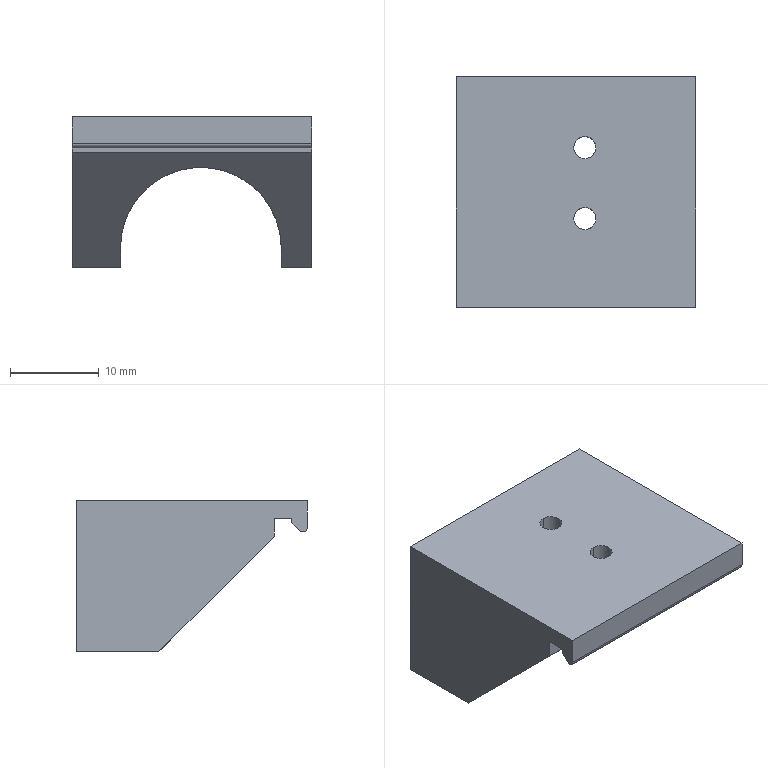NC program | NX | posted with a generic post | part box 27 x 26 x 17 mm
Lines 2084 to 2885 of 22937:
(FIXED_CONTOUR , TOOL : R2)
N4124 T03 M6
N4126 G54
N4128 G17 G0 G90 X-4.906 Y-8.76 S9500 M3
N4130 G43 Z30. H3
N4132 Z-6.
N4134 G94 G1 Z-9.999 F1000.
N4136 G3 X-5.01 Y-8.374 R0.4
N4138 G1 X-5.17 Y-8.214 Z-9.884 F3000.
N4140 X-5.387 Y-7.997 Z-9.717
N4142 X-5.602 Y-7.782 Z-9.538
N4144 X-5.786 Y-7.598 Z-9.376
N4146 X-6.018 Y-7.366 Z-9.151
N4148 X-6.185 Y-7.199 Z-8.977
N4150 X-6.356 Y-7.028 Z-8.783
N4152 X-6.385 Y-6.998 Z-8.747
N4154 X-6.526 Y-6.81 Z-8.578
N4156 X-6.336 Y-7. Z-8.805
N4158 X-6.185 Y-7.151 Z-8.977
N4160 X-6.014 Y-7.322 Z-9.156
N4162 X-5.786 Y-7.55 Z-9.376
N4164 X-5.583 Y-7.752 Z-9.553
N4166 X-5.387 Y-7.949 Z-9.717
N4168 X-5.154 Y-8.182 Z-9.895
N4170 X-4.988 Y-8.348 Z-10.014
N4172 X-4.856 Y-8.48 Z-10.099
N4174 X-4.75 Y-8.551 Z-10.166
N4176 X-4.988 Y-8.313 Z-10.014
N4178 X-5.143 Y-8.158 Z-9.903
N4180 X-5.387 Y-7.914 Z-9.717
N4182 X-5.57 Y-7.731 Z-9.565
N4184 X-5.786 Y-7.515 Z-9.376
N4186 X-6.01 Y-7.29 Z-9.159
N4188 X-6.185 Y-7.116 Z-8.977
N4190 X-6.362 Y-6.938 Z-8.775
N4192 X-6.507 Y-6.794 Z-8.6
N4194 X-6.601 Y-6.7 Z-8.481
N4196 X-6.64 Y-6.643 Z-8.43
N4198 X-6.665 Y-6.603 Z-8.394
N4200 X-6.638 Y-6.63 Z-8.432
N4202 X-6.492 Y-6.776 Z-8.618
N4204 X-6.365 Y-6.903 Z-8.772
N4206 X-6.185 Y-7.084 Z-8.977
N4208 X-6.007 Y-7.261 Z-9.162
N4210 X-5.786 Y-7.482 Z-9.376
N4212 X-5.557 Y-7.711 Z-9.575
N4214 X-5.387 Y-7.881 Z-9.717
N4216 X-5.132 Y-8.136 Z-9.911
N4218 X-4.989 Y-8.279 Z-10.013
N4220 X-4.65 Y-8.618 Z-10.229
N4222 X-4.556 Y-8.679 Z-10.286
N4224 X-4.621 Y-8.615 Z-10.248
N4226 X-4.988 Y-8.247 Z-10.014
N4228 X-5.121 Y-8.114 Z-9.919
N4230 X-5.387 Y-7.848 Z-9.717
N4232 X-5.544 Y-7.691 Z-9.586
N4234 X-5.786 Y-7.449 Z-9.376
N4236 X-6.004 Y-7.231 Z-9.166
N4238 X-6.185 Y-7.051 Z-8.977
N4240 X-6.368 Y-6.868 Z-8.769
N4242 X-6.478 Y-6.758 Z-8.636
N4244 X-6.634 Y-6.601 Z-8.438
N4246 X-6.72 Y-6.516 Z-8.316
N4248 X-6.779 Y-6.421 Z-8.231
N4250 X-6.63 Y-6.57 Z-8.443
N4252 X-6.461 Y-6.738 Z-8.656
N4254 X-6.37 Y-6.829 Z-8.766
N4256 X-6.185 Y-7.015 Z-8.977
N4258 X-6.001 Y-7.198 Z-9.169
N4260 X-5.786 Y-7.414 Z-9.376
N4262 X-5.53 Y-7.669 Z-9.598
N4264 X-5.387 Y-7.812 Z-9.717
N4266 X-5.109 Y-8.09 Z-9.927
N4268 X-4.988 Y-8.211 Z-10.014
N4270 X-4.589 Y-8.61 Z-10.267
N4272 X-4.541 Y-8.658 Z-10.293
N4274 X-4.461 Y-8.738 Z-10.341
N4276 X-4.37 Y-8.793 Z-10.392
N4278 X-4.408 Y-8.755 Z-10.371
N4280 X-4.507 Y-8.657 Z-10.312
N4282 X-4.615 Y-8.548 Z-10.252
N4284 X-4.988 Y-8.175 Z-10.014
N4286 X-5.097 Y-8.066 Z-9.936
N4288 X-5.387 Y-7.776 Z-9.717
N4290 X-5.516 Y-7.647 Z-9.61
N4292 X-5.786 Y-7.377 Z-9.376
N4294 X-5.998 Y-7.166 Z-9.173
N4296 X-6.185 Y-6.979 Z-8.977
N4298 X-6.373 Y-6.79 Z-8.762
N4300 X-6.445 Y-6.718 Z-8.676
N4302 X-6.625 Y-6.538 Z-8.449
N4304 X-6.834 Y-6.329 Z-8.152
N4306 X-6.89 Y-6.237 Z-8.072
N4308 X-6.62 Y-6.506 Z-8.455
N4310 X-6.428 Y-6.698 Z-8.696
N4312 X-6.376 Y-6.75 Z-8.759
N4314 X-6.185 Y-6.942 Z-8.977
N4316 X-5.994 Y-7.132 Z-9.176
N4318 X-5.786 Y-7.34 Z-9.376
N4320 X-5.502 Y-7.624 Z-9.622
N4322 X-5.387 Y-7.739 Z-9.717
N4324 X-5.085 Y-8.041 Z-9.945
N4326 X-4.988 Y-8.138 Z-10.014
N4328 X-4.589 Y-8.537 Z-10.267
N4330 X-4.471 Y-8.655 Z-10.332
N4332 X-4.384 Y-8.742 Z-10.384
N4334 X-4.288 Y-8.838 Z-10.435
N4336 X-4.198 Y-8.888 Z-10.483
N4338 X-4.358 Y-8.728 Z-10.398
N4340 X-4.433 Y-8.653 Z-10.353
N4342 X-4.609 Y-8.477 Z-10.255
N4344 X-4.988 Y-8.098 Z-10.014
N4346 X-5.072 Y-8.014 Z-9.954
N4348 X-5.387 Y-7.699 Z-9.717
N4350 X-5.486 Y-7.599 Z-9.635
N4352 X-5.786 Y-7.3 Z-9.376
N4354 X-5.99 Y-7.095 Z-9.18
N4356 X-6.185 Y-6.901 Z-8.977
N4358 X-6.379 Y-6.706 Z-8.755
N4360 X-6.615 Y-6.47 Z-8.462
N4362 X-6.876 Y-6.21 Z-8.093
N4364 X-6.944 Y-6.142 Z-7.989
N4366 X-7.001 Y-6.037 Z-7.898
N4368 X-6.982 Y-6.056 Z-7.93
N4370 X-6.866 Y-6.172 Z-8.107
N4372 X-6.793 Y-6.245 Z-8.208
N4374 X-6.609 Y-6.429 Z-8.469
N4376 X-6.383 Y-6.655 Z-8.751
N4378 X-6.185 Y-6.854 Z-8.977
N4380 X-5.986 Y-7.052 Z-9.185
N4382 X-5.786 Y-7.253 Z-9.376
N4384 X-5.468 Y-7.57 Z-9.65
N4386 X-5.387 Y-7.651 Z-9.717
N4388 X-5.057 Y-7.982 Z-9.965
N4390 X-4.988 Y-8.05 Z-10.014
N4392 X-4.589 Y-8.449 Z-10.267
N4394 X-4.388 Y-8.65 Z-10.378
N4396 X-4.327 Y-8.712 Z-10.414
N4398 X-4.19 Y-8.848 Z-10.487
N4400 X-4.101 Y-8.937 Z-10.529
N4402 X-4.01 Y-8.983 Z-10.573
N4404 X-4.19 Y-8.802 Z-10.487
N4406 X-4.297 Y-8.696 Z-10.43
N4408 X-4.345 Y-8.648 Z-10.402
N4410 X-4.602 Y-8.391 Z-10.259
N4412 X-4.988 Y-8.005 Z-10.014
N4414 X-5.042 Y-7.951 Z-9.976
N4416 X-5.387 Y-7.606 Z-9.718
N4418 X-5.45 Y-7.542 Z-9.665
N4420 X-5.786 Y-7.207 Z-9.377
N4422 X-5.985 Y-7.008 Z-9.186
N4424 X-6.185 Y-6.808 Z-8.977
N4426 X-6.384 Y-6.609 Z-8.75
N4428 X-6.604 Y-6.389 Z-8.477
N4430 X-6.747 Y-6.245 Z-8.272
N4432 X-6.857 Y-6.136 Z-8.121
N4434 X-6.982 Y-6.011 Z-7.93
N4436 X-7.049 Y-5.944 Z-7.818
N4438 X-7.094 Y-5.855 Z-7.742
N4440 X-6.982 Y-5.966 Z-7.93
N4442 X-6.848 Y-6.101 Z-8.135
N4444 X-6.703 Y-6.245 Z-8.335
N4446 X-6.583 Y-6.365 Z-8.503
N4448 X-6.384 Y-6.565 Z-8.75
N4450 X-6.185 Y-6.764 Z-8.977
N4452 X-5.985 Y-6.963 Z-9.186
N4454 X-5.786 Y-7.163 Z-9.377
N4456 X-5.387 Y-7.562 Z-9.718
N4458 X-4.988 Y-7.96 Z-10.014
N4460 X-4.589 Y-8.359 Z-10.267
N4462 X-4.303 Y-8.646 Z-10.425
N4464 X-4.268 Y-8.681 Z-10.445
N4466 X-4.19 Y-8.758 Z-10.487
N4468 X-3.921 Y-9.028 Z-10.616
N4470 X-3.831 Y-9.072 Z-10.656
N4472 X-3.898 Y-9.005 Z-10.627
N4474 X-4.19 Y-8.713 Z-10.487
N4476 X-4.595 Y-8.308 Z-10.263
N4478 X-4.988 Y-7.915 Z-10.015
N4480 X-5.387 Y-7.516 Z-9.718
N4482 X-5.786 Y-7.118 Z-9.377
N4484 X-5.985 Y-6.918 Z-9.186
N4486 X-6.185 Y-6.719 Z-8.977
N4488 X-6.384 Y-6.519 Z-8.751
N4490 X-6.593 Y-6.311 Z-8.491
N4492 X-6.658 Y-6.245 Z-8.398
N4494 X-6.839 Y-6.065 Z-8.148
N4496 X-6.982 Y-5.921 Z-7.93
N4498 X-7.104 Y-5.799 Z-7.725
N4500 X-7.135 Y-5.768 Z-7.666
N4502 X-7.178 Y-5.679 Z-7.589
N4504 X-7.108 Y-5.748 Z-7.717
N4506 X-6.982 Y-5.874 Z-7.93
N4508 X-6.829 Y-6.027 Z-8.162
N4510 X-6.583 Y-6.273 Z-8.503
N4512 X-6.384 Y-6.473 Z-8.751
N4514 X-6.185 Y-6.672 Z-8.978
N4516 X-5.985 Y-6.871 Z-9.186
N4518 X-5.786 Y-7.071 Z-9.377
N4520 X-5.387 Y-7.47 Z-9.718
N4522 X-4.988 Y-7.868 Z-10.015
N4524 X-4.591 Y-8.265 Z-10.265
N4526 X-4.19 Y-8.666 Z-10.486
N4528 X-3.887 Y-8.969 Z-10.631
N4530 X-3.741 Y-9.115 Z-10.695
N4532 X-3.652 Y-9.156 Z-10.732
N4534 X-3.723 Y-9.085 Z-10.701
N4536 X-3.792 Y-9.016 Z-10.674
N4538 X-3.877 Y-8.931 Z-10.636
N4540 X-4.19 Y-8.618 Z-10.486
N4542 X-4.589 Y-8.219 Z-10.267
N4544 X-4.988 Y-7.82 Z-10.015
N4546 X-5.387 Y-7.421 Z-9.718
N4548 X-5.786 Y-7.022 Z-9.377
N4550 X-5.985 Y-6.823 Z-9.186
N4552 X-6.185 Y-6.624 Z-8.978
N4554 X-6.384 Y-6.424 Z-8.751
N4556 X-6.583 Y-6.225 Z-8.503
N4558 X-6.819 Y-5.989 Z-8.177
N4560 X-6.982 Y-5.826 Z-7.93
N4562 X-7.113 Y-5.695 Z-7.709
N4564 X-7.221 Y-5.587 Z-7.509
N4566 X-7.265 Y-5.491 Z-7.428
N4568 X-7.118 Y-5.638 Z-7.701
N4570 X-6.982 Y-5.774 Z-7.93
N4572 X-6.809 Y-5.948 Z-8.193
N4574 X-6.583 Y-6.173 Z-8.503
N4576 X-6.384 Y-6.372 Z-8.751
N4578 X-6.185 Y-6.572 Z-8.978
N4580 X-5.985 Y-6.771 Z-9.187
N4582 X-5.786 Y-6.971 Z-9.377
N4584 X-5.387 Y-7.369 Z-9.718
N4586 X-4.988 Y-7.768 Z-10.015
N4588 X-4.589 Y-8.167 Z-10.267
N4590 X-4.19 Y-8.566 Z-10.487
N4592 X-3.865 Y-8.891 Z-10.641
N4594 X-3.792 Y-8.965 Z-10.674
N4596 X-3.678 Y-9.079 Z-10.719
N4598 X-3.6 Y-9.157 Z-10.753
N4600 X-3.56 Y-9.196 Z-10.769
N4602 X-3.464 Y-9.236 Z-10.805
N4604 X-3.563 Y-9.136 Z-10.767
N4606 X-3.627 Y-9.072 Z-10.739
N4608 X-3.792 Y-8.907 Z-10.674
N4610 X-3.852 Y-8.847 Z-10.647
N4612 X-4.19 Y-8.509 Z-10.487
N4614 X-4.589 Y-8.11 Z-10.267
N4616 X-4.988 Y-7.711 Z-10.015
N4618 X-5.387 Y-7.312 Z-9.718
N4620 X-5.786 Y-6.913 Z-9.377
N4622 X-5.985 Y-6.714 Z-9.187
N4624 X-6.185 Y-6.515 Z-8.978
N4626 X-6.384 Y-6.315 Z-8.751
N4628 X-6.583 Y-6.116 Z-8.504
N4630 X-6.797 Y-5.902 Z-8.21
N4632 X-6.982 Y-5.717 Z-7.93
N4634 X-7.123 Y-5.576 Z-7.691
N4636 X-7.28 Y-5.419 Z-7.402
N4638 X-7.31 Y-5.389 Z-7.34
N4640 X-7.351 Y-5.293 Z-7.256
N4642 X-7.268 Y-5.375 Z-7.424
N4644 X-7.129 Y-5.514 Z-7.682
N4646 X-6.982 Y-5.661 Z-7.93
N4648 X-6.786 Y-5.858 Z-8.227
N4650 X-6.583 Y-6.06 Z-8.504
N4652 X-6.384 Y-6.259 Z-8.752
N4654 X-6.185 Y-6.459 Z-8.978
N4656 X-5.985 Y-6.658 Z-9.187
N4658 X-5.786 Y-6.858 Z-9.378
N4660 X-5.387 Y-7.256 Z-9.719
N4662 X-4.988 Y-7.655 Z-10.015
N4664 X-4.589 Y-8.054 Z-10.267
N4666 X-4.19 Y-8.453 Z-10.487
N4668 X-3.792 Y-8.852 Z-10.674
N4670 X-3.578 Y-9.065 Z-10.758
N4672 X-3.527 Y-9.116 Z-10.781
N4674 X-3.37 Y-9.273 Z-10.84
N4676 X-3.286 Y-9.304 Z-10.869
N4678 X-3.393 Y-9.197 Z-10.832
N4680 X-3.494 Y-9.096 Z-10.794
N4682 X-3.532 Y-9.058 Z-10.777
N4684 X-3.792 Y-8.798 Z-10.674
N4686 X-4.19 Y-8.399 Z-10.487
N4688 X-4.589 Y-8.001 Z-10.267
N4690 X-4.988 Y-7.602 Z-10.015
N4692 X-5.387 Y-7.203 Z-9.719
N4694 X-5.786 Y-6.804 Z-9.378
N4696 X-5.985 Y-6.605 Z-9.187
N4698 X-6.185 Y-6.405 Z-8.979
N4700 X-6.384 Y-6.206 Z-8.752
N4702 X-6.583 Y-6.007 Z-8.504
N4704 X-6.783 Y-5.807 Z-8.232
N4706 X-6.982 Y-5.608 Z-7.93
N4708 X-7.134 Y-5.456 Z-7.674
N4710 X-7.257 Y-5.333 Z-7.445
N4712 X-7.381 Y-5.209 Z-7.193
N4714 X-7.388 Y-5.202 Z-7.179
N4716 X-7.422 Y-5.115 Z-7.106
N4718 X-7.348 Y-5.189 Z-7.262
N4720 X-7.246 Y-5.291 Z-7.466
N4722 X-7.122 Y-5.415 Z-7.693
N4724 X-6.982 Y-5.555 Z-7.931
N4726 X-6.783 Y-5.754 Z-8.232
N4728 X-6.583 Y-5.954 Z-8.504
N4730 X-6.384 Y-6.153 Z-8.752
N4732 X-6.185 Y-6.352 Z-8.979
N4734 X-5.985 Y-6.552 Z-9.188
N4736 X-5.786 Y-6.751 Z-9.378
N4738 X-5.387 Y-7.15 Z-9.719
N4740 X-4.988 Y-7.549 Z-10.016
N4742 X-4.589 Y-7.948 Z-10.268
N4744 X-4.19 Y-8.346 Z-10.487
N4746 X-3.792 Y-8.745 Z-10.674
N4748 X-3.393 Y-9.144 Z-10.832
N4750 X-3.202 Y-9.334 Z-10.898
N4752 X-3.118 Y-9.365 Z-10.927
N4754 X-3.426 Y-9.058 Z-10.819
N4756 X-3.803 Y-8.68 Z-10.669
N4758 X-4.19 Y-8.293 Z-10.487
N4760 X-4.589 Y-7.894 Z-10.268
N4762 X-4.988 Y-7.495 Z-10.016
N4764 X-5.387 Y-7.097 Z-9.719
N4766 X-5.786 Y-6.698 Z-9.378
N4768 X-5.985 Y-6.498 Z-9.188
N4770 X-6.185 Y-6.299 Z-8.979
N4772 X-6.384 Y-6.1 Z-8.752
N4774 X-6.583 Y-5.9 Z-8.505
N4776 X-6.783 Y-5.701 Z-8.232
N4778 X-6.982 Y-5.501 Z-7.931
N4780 X-7.148 Y-5.336 Z-7.649
N4782 X-7.235 Y-5.249 Z-7.488
N4784 X-7.382 Y-5.101 Z-7.191
N4786 X-7.455 Y-5.028 Z-7.033
N4788 X-7.486 Y-4.941 Z-6.958
N4790 X-7.439 Y-4.987 Z-7.069
N4792 X-7.381 Y-5.045 Z-7.193
N4794 X-7.223 Y-5.204 Z-7.51
N4796 X-7.155 Y-5.271 Z-7.635
N4798 X-6.982 Y-5.444 Z-7.931
N4800 X-6.783 Y-5.644 Z-8.233
N4802 X-6.583 Y-5.843 Z-8.505
N4804 X-6.384 Y-6.043 Z-8.752
N4806 X-6.185 Y-6.242 Z-8.979
N4808 X-5.985 Y-6.441 Z-9.188
N4810 X-5.786 Y-6.641 Z-9.379
N4812 X-5.387 Y-7.04 Z-9.719
N4814 X-4.988 Y-7.438 Z-10.016
N4816 X-4.589 Y-7.837 Z-10.268
N4818 X-4.19 Y-8.236 Z-10.487
N4820 X-3.792 Y-8.635 Z-10.674
N4822 X-3.393 Y-9.034 Z-10.832
N4824 X-3.028 Y-9.398 Z-10.958
N4826 X-2.936 Y-9.429 Z-10.989
N4828 X-3.393 Y-8.973 Z-10.832
N4830 X-3.792 Y-8.574 Z-10.674
N4832 X-4.19 Y-8.175 Z-10.487
N4834 X-4.589 Y-7.776 Z-10.268
N4836 X-4.988 Y-7.378 Z-10.016
N4838 X-5.387 Y-6.979 Z-9.72
N4840 X-5.786 Y-6.58 Z-9.379
N4842 X-5.985 Y-6.381 Z-9.188
N4844 X-6.185 Y-6.181 Z-8.979
N4846 X-6.384 Y-5.982 Z-8.753
N4848 X-6.583 Y-5.782 Z-8.505
N4850 X-6.783 Y-5.583 Z-8.233
N4852 X-6.982 Y-5.384 Z-7.931
N4854 X-7.163 Y-5.202 Z-7.621
N4856 X-7.21 Y-5.156 Z-7.535
N4858 X-7.381 Y-4.985 Z-7.193
N4860 X-7.43 Y-4.935 Z-7.088
N4862 X-7.519 Y-4.847 Z-6.878
N4864 X-7.553 Y-4.748 Z-6.795
N4866 X-7.421 Y-4.88 Z-7.109
N4868 X-7.381 Y-4.919 Z-7.193
N4870 X-7.196 Y-5.104 Z-7.561
N4872 X-7.172 Y-5.128 Z-7.606
N4874 X-6.982 Y-5.318 Z-7.932
N4876 X-6.783 Y-5.518 Z-8.233
N4878 X-6.583 Y-5.717 Z-8.506
N4880 X-6.384 Y-5.916 Z-8.753
N4882 X-6.185 Y-6.116 Z-8.98
N4884 X-5.985 Y-6.315 Z-9.189
N4886 X-5.786 Y-6.515 Z-9.379
N4888 X-5.387 Y-6.913 Z-9.72
N4890 X-4.988 Y-7.312 Z-10.017
N4892 X-4.589 Y-7.711 Z-10.268
N4894 X-4.19 Y-8.11 Z-10.488
N4896 X-3.792 Y-8.509 Z-10.674
N4898 X-3.393 Y-8.907 Z-10.832
N4900 X-2.994 Y-9.306 Z-10.969
N4902 X-2.937 Y-9.363 Z-10.986
N4904 X-2.902 Y-9.398 Z-10.998
N4906 X-2.842 Y-9.458 Z-11.015
N4908 X-2.755 Y-9.485 Z-11.038
N4910 X-2.875 Y-9.366 Z-11.006
N4912 X-2.906 Y-9.334 Z-10.995
N4914 X-2.994 Y-9.246 Z-10.969
N4916 X-3.393 Y-8.847 Z-10.832
N4918 X-3.792 Y-8.449 Z-10.674
N4920 X-4.19 Y-8.05 Z-10.488
N4922 X-4.589 Y-7.651 Z-10.269
N4924 X-4.988 Y-7.252 Z-10.017
N4926 X-5.387 Y-6.853 Z-9.72
N4928 X-5.786 Y-6.454 Z-9.379
N4930 X-5.985 Y-6.255 Z-9.189
N4932 X-6.185 Y-6.056 Z-8.98
N4934 X-6.384 Y-5.856 Z-8.753
N4936 X-6.583 Y-5.657 Z-8.506
N4938 X-6.783 Y-5.457 Z-8.234
N4940 X-6.982 Y-5.258 Z-7.932
N4942 X-7.184 Y-5.056 Z-7.585
N4944 X-7.381 Y-4.859 Z-7.194
N4946 X-7.412 Y-4.828 Z-7.128
N4948 X-7.584 Y-4.657 Z-6.719
N4950 X-7.609 Y-4.572 Z-6.647
N4952 X-7.582 Y-4.6 Z-6.724
N4954 X-7.403 Y-4.778 Z-7.146
N4956 X-7.381 Y-4.8 Z-7.194
N4958 X-7.182 Y-5. Z-7.589
N4960 X-6.982 Y-5.199 Z-7.932
N4962 X-6.783 Y-5.399 Z-8.234
N4964 X-6.583 Y-5.598 Z-8.506
N4966 X-6.384 Y-5.797 Z-8.754
N4968 X-6.185 Y-5.997 Z-8.98
N4970 X-5.985 Y-6.196 Z-9.189
N4972 X-5.786 Y-6.396 Z-9.38
N4974 X-5.387 Y-6.794 Z-9.72
N4976 X-4.988 Y-7.193 Z-10.017
N4978 X-4.589 Y-7.592 Z-10.269
N4980 X-4.19 Y-7.991 Z-10.488
N4982 X-3.792 Y-8.39 Z-10.675
N4984 X-3.393 Y-8.789 Z-10.832
N4986 X-2.994 Y-9.187 Z-10.969
N4988 X-2.876 Y-9.305 Z-11.003
N4990 X-2.848 Y-9.334 Z-11.013
N4992 X-2.67 Y-9.511 Z-11.061
N4994 X-2.587 Y-9.536 Z-11.083
N4996 X-2.821 Y-9.303 Z-11.02
N4998 X-2.846 Y-9.277 Z-11.011
N5000 X-2.994 Y-9.129 Z-10.968
N5002 X-3.393 Y-8.731 Z-10.832
N5004 X-3.792 Y-8.332 Z-10.675
N5006 X-4.19 Y-7.933 Z-10.488
N5008 X-4.589 Y-7.534 Z-10.269
N5010 X-4.988 Y-7.135 Z-10.017
N5012 X-5.387 Y-6.736 Z-9.721
N5014 X-5.786 Y-6.338 Z-9.38
N5016 X-5.985 Y-6.138 Z-9.189
N5018 X-6.185 Y-5.939 Z-8.981
N5020 X-6.384 Y-5.739 Z-8.754
N5022 X-6.583 Y-5.54 Z-8.506
N5024 X-6.783 Y-5.341 Z-8.234
N5026 X-6.982 Y-5.141 Z-7.932
N5028 X-7.182 Y-4.942 Z-7.589
N5030 X-7.395 Y-4.729 Z-7.164
N5032 X-7.475 Y-4.649 Z-6.975
N5034 X-7.576 Y-4.548 Z-6.739
N5036 X-7.634 Y-4.489 Z-6.577
N5038 X-7.658 Y-4.408 Z-6.508
N5040 X-7.57 Y-4.496 Z-6.754
N5042 X-7.381 Y-4.685 Z-7.194
N5044 X-7.182 Y-4.885 Z-7.59
N5046 X-6.982 Y-5.084 Z-7.933
N5048 X-6.783 Y-5.283 Z-8.235
N5050 X-6.583 Y-5.483 Z-8.507
N5052 X-6.384 Y-5.682 Z-8.754
N5054 X-6.185 Y-5.882 Z-8.981
N5056 X-5.985 Y-6.081 Z-9.19
N5058 X-5.786 Y-6.28 Z-9.38
N5060 X-5.387 Y-6.679 Z-9.721
N5062 X-4.988 Y-7.078 Z-10.017
N5064 X-4.589 Y-7.477 Z-10.269
N5066 X-4.19 Y-7.876 Z-10.488
N5068 X-3.792 Y-8.274 Z-10.675
N5070 X-3.393 Y-8.673 Z-10.832
N5072 X-2.994 Y-9.072 Z-10.968
N5074 X-2.794 Y-9.272 Z-11.027
N5076 X-2.595 Y-9.471 Z-11.082
N5078 X-2.511 Y-9.556 Z-11.099
N5080 X-2.434 Y-9.575 Z-11.114
N5082 X-2.595 Y-9.413 Z-11.082
N5084 X-2.768 Y-9.241 Z-11.035
N5086 X-2.994 Y-9.015 Z-10.968
N5088 X-3.393 Y-8.616 Z-10.832
N5090 X-3.792 Y-8.217 Z-10.675
N5092 X-4.19 Y-7.818 Z-10.489
N5094 X-4.589 Y-7.419 Z-10.269
N5096 X-4.988 Y-7.021 Z-10.018
N5098 X-5.387 Y-6.622 Z-9.721
N5100 X-5.786 Y-6.223 Z-9.38
N5102 X-5.985 Y-6.024 Z-9.19
N5104 X-6.185 Y-5.824 Z-8.981
N5106 X-6.384 Y-5.625 Z-8.754
N5108 X-6.583 Y-5.425 Z-8.507
N5110 X-6.783 Y-5.226 Z-8.235
N5112 X-6.982 Y-5.026 Z-7.933
N5114 X-7.182 Y-4.827 Z-7.59
N5116 X-7.381 Y-4.628 Z-7.194
N5118 X-7.564 Y-4.444 Z-6.768
N5120 X-7.682 Y-4.327 Z-6.441
N5122 X-7.705 Y-4.246 Z-6.373
N5124 X-7.558 Y-4.392 Z-6.783
N5126 X-7.381 Y-4.57 Z-7.194
N5128 X-7.182 Y-4.769 Z-7.59
N5130 X-6.982 Y-4.969 Z-7.933
N5132 X-6.783 Y-5.168 Z-8.235
N5134 X-6.583 Y-5.368 Z-8.507
N5136 X-6.384 Y-5.567 Z-8.755
N5138 X-6.185 Y-5.766 Z-8.982
N5140 X-5.985 Y-5.966 Z-9.19
N5142 X-5.786 Y-6.165 Z-9.381
N5144 X-5.387 Y-6.564 Z-9.722
N5146 X-4.988 Y-6.963 Z-10.018
N5148 X-4.589 Y-7.362 Z-10.27
N5150 X-4.19 Y-7.76 Z-10.489
N5152 X-3.792 Y-8.159 Z-10.675
N5154 X-3.393 Y-8.558 Z-10.832
N5156 X-2.994 Y-8.957 Z-10.968
N5158 X-2.741 Y-9.21 Z-11.042
N5160 X-2.595 Y-9.356 Z-11.082
N5162 X-2.361 Y-9.59 Z-11.129
N5164 X-2.286 Y-9.604 Z-11.144
N5166 X-2.595 Y-9.295 Z-11.082
N5168 X-2.727 Y-9.164 Z-11.045
N5170 X-2.994 Y-8.896 Z-10.968
N5172 X-3.393 Y-8.497 Z-10.833
N5174 X-3.792 Y-8.099 Z-10.675
N5176 X-4.19 Y-7.7 Z-10.489
N5178 X-4.589 Y-7.301 Z-10.27
N5180 X-4.988 Y-6.902 Z-10.019
N5182 X-5.387 Y-6.503 Z-9.722
N5184 X-5.786 Y-6.105 Z-9.382
N5186 X-5.985 Y-5.905 Z-9.19
N5188 X-6.185 Y-5.706 Z-8.982
N5190 X-6.384 Y-5.506 Z-8.755
N5192 X-6.583 Y-5.307 Z-8.507
N5194 X-6.783 Y-5.108 Z-8.235
N5196 X-6.982 Y-4.908 Z-7.934
N5198 X-7.182 Y-4.709 Z-7.591
N5200 X-7.381 Y-4.509 Z-7.195
N5202 X-7.552 Y-4.338 Z-6.798
N5204 X-7.701 Y-4.189 Z-6.387
N5206 X-7.727 Y-4.164 Z-6.305
N5208 X-7.749 Y-4.078 Z-6.232
N5210 X-7.697 Y-4.129 Z-6.399
N5212 X-7.546 Y-4.281 Z-6.814
N5214 X-7.381 Y-4.446 Z-7.195
N5216 X-7.182 Y-4.645 Z-7.591
N5218 X-6.982 Y-4.845 Z-7.934
N5220 X-6.783 Y-5.044 Z-8.236
N5222 X-6.583 Y-5.243 Z-8.508
N5224 X-6.384 Y-5.443 Z-8.755
N5226 X-6.185 Y-5.642 Z-8.983
N5228 X-5.985 Y-5.842 Z-9.191
N5230 X-5.786 Y-6.041 Z-9.382
N5232 X-5.387 Y-6.44 Z-9.723
N5234 X-4.988 Y-6.839 Z-10.019
N5236 X-4.589 Y-7.237 Z-10.27
N5238 X-4.19 Y-7.636 Z-10.489
N5240 X-3.792 Y-8.035 Z-10.676
N5242 X-3.393 Y-8.434 Z-10.833
N5244 X-2.994 Y-8.833 Z-10.968
N5246 X-2.595 Y-9.231 Z-11.082
N5248 X-2.207 Y-9.62 Z-11.16
N5250 X-2.128 Y-9.632 Z-11.172
N5252 X-2.196 Y-9.563 Z-11.162
N5254 X-2.595 Y-9.164 Z-11.081
N5256 X-2.994 Y-8.766 Z-10.968
N5258 X-3.393 Y-8.367 Z-10.833
N5260 X-3.792 Y-7.968 Z-10.676
N5262 X-4.19 Y-7.569 Z-10.489
N5264 X-4.589 Y-7.17 Z-10.271
N5266 X-4.988 Y-6.772 Z-10.02
N5268 X-5.387 Y-6.373 Z-9.724
N5270 X-5.786 Y-5.974 Z-9.383
N5272 X-5.985 Y-5.775 Z-9.192
N5274 X-6.185 Y-5.575 Z-8.983
N5276 X-6.384 Y-5.376 Z-8.756
N5278 X-6.583 Y-5.176 Z-8.508
N5280 X-6.783 Y-4.977 Z-8.236
N5282 X-6.982 Y-4.778 Z-7.934
N5284 X-7.182 Y-4.578 Z-7.592
N5286 X-7.381 Y-4.379 Z-7.196
N5288 X-7.546 Y-4.214 Z-6.815
N5290 X-7.693 Y-4.066 Z-6.411
N5292 X-7.772 Y-3.988 Z-6.158
N5294 X-7.794 Y-3.893 Z-6.079
N5296 X-7.78 Y-3.907 Z-6.132
N5298 X-7.689 Y-3.997 Z-6.424
N5300 X-7.554 Y-4.133 Z-6.796
N5302 X-7.381 Y-4.305 Z-7.196
N5304 X-7.182 Y-4.505 Z-7.592
N5306 X-6.982 Y-4.704 Z-7.935
N5308 X-6.783 Y-4.904 Z-8.236
N5310 X-6.583 Y-5.103 Z-8.508
N5312 X-6.384 Y-5.302 Z-8.757
N5314 X-6.185 Y-5.502 Z-8.984
N5316 X-5.985 Y-5.701 Z-9.193
N5318 X-5.786 Y-5.901 Z-9.384
N5320 X-5.387 Y-6.299 Z-9.725
N5322 X-4.988 Y-6.698 Z-10.02
N5324 X-4.589 Y-7.097 Z-10.271
N5326 X-4.19 Y-7.496 Z-10.49
N5328 X-3.792 Y-7.895 Z-10.676
N5330 X-3.393 Y-8.293 Z-10.833
N5332 X-2.994 Y-8.692 Z-10.968
N5334 X-2.595 Y-9.091 Z-11.081
N5336 X-2.196 Y-9.49 Z-11.162
N5338 X-2.043 Y-9.643 Z-11.185
N5340 X-1.961 Y-9.655 Z-11.197
N5342 X-2.196 Y-9.419 Z-11.162
N5344 X-2.595 Y-9.02 Z-11.081
N5346 X-2.994 Y-8.622 Z-10.969
N5348 X-3.393 Y-8.223 Z-10.833
N5350 X-3.792 Y-7.824 Z-10.676
N5352 X-4.19 Y-7.425 Z-10.49
N5354 X-4.589 Y-7.026 Z-10.272
N5356 X-4.988 Y-6.628 Z-10.021
N5358 X-5.387 Y-6.229 Z-9.726
N5360 X-5.786 Y-5.83 Z-9.384
N5362 X-5.985 Y-5.631 Z-9.195
N5364 X-6.2 Y-5.415 Z-8.966
N5366 X-6.384 Y-5.232 Z-8.758
N5368 X-6.583 Y-5.032 Z-8.509
N5370 X-6.783 Y-4.833 Z-8.237
N5372 X-6.982 Y-4.634 Z-7.935
N5374 X-7.182 Y-4.434 Z-7.593
N5376 X-7.381 Y-4.235 Z-7.197
N5378 X-7.561 Y-4.055 Z-6.778
N5380 X-7.685 Y-3.931 Z-6.437
N5382 X-7.78 Y-3.836 Z-6.132
N5384 X-7.812 Y-3.803 Z-6.005
N5386 X-7.83 Y-3.717 Z-5.934
N5388 X-7.78 Y-3.767 Z-6.132
N5390 X-7.681 Y-3.866 Z-6.45
N5392 X-7.568 Y-3.979 Z-6.761
N5394 X-7.381 Y-4.166 Z-7.197
N5396 X-7.182 Y-4.365 Z-7.593
N5398 X-6.982 Y-4.565 Z-7.935
N5400 X-6.783 Y-4.764 Z-8.237
N5402 X-6.583 Y-4.964 Z-8.51
N5404 X-6.384 Y-5.163 Z-8.759
N5406 X-6.185 Y-5.362 Z-8.986
N5408 X-5.985 Y-5.562 Z-9.196
N5410 X-5.786 Y-5.761 Z-9.386
N5412 X-5.387 Y-6.16 Z-9.727
N5414 X-4.988 Y-6.559 Z-10.023
N5416 X-4.589 Y-6.958 Z-10.273
N5418 X-4.19 Y-7.356 Z-10.491
N5420 X-3.792 Y-7.755 Z-10.677
N5422 X-3.393 Y-8.154 Z-10.834
N5424 X-2.994 Y-8.553 Z-10.969
N5426 X-2.595 Y-8.952 Z-11.082
N5428 X-2.196 Y-9.35 Z-11.162
N5430 X-1.881 Y-9.666 Z-11.208
N5432 X-1.803 Y-9.677 Z-11.22
N5434 X-2.196 Y-9.283 Z-11.162
N5436 X-2.595 Y-8.885 Z-11.082
N5438 X-2.994 Y-8.486 Z-10.969
N5440 X-3.393 Y-8.087 Z-10.834
N5442 X-3.792 Y-7.688 Z-10.678
N5444 X-4.19 Y-7.289 Z-10.492
N5446 X-4.589 Y-6.89 Z-10.275
N5448 X-4.988 Y-6.492 Z-10.024
N5450 X-5.387 Y-6.093 Z-9.729
N5452 X-5.786 Y-5.694 Z-9.388
N5454 X-5.985 Y-5.495 Z-9.197
N5456 X-6.185 Y-5.295 Z-8.988
N5458 X-6.384 Y-5.096 Z-8.76
N5460 X-6.583 Y-4.896 Z-8.512
N5462 X-6.783 Y-4.697 Z-8.237
N5464 X-6.932 Y-4.548 Z-8.014
N5466 X-6.982 Y-4.498 Z-7.936
N5468 X-7.182 Y-4.298 Z-7.593
N5470 X-7.381 Y-4.099 Z-7.198
N5472 X-7.575 Y-3.904 Z-6.744
N5474 X-7.68 Y-3.8 Z-6.453
N5476 X-7.78 Y-3.7 Z-6.133
N5478 X-7.847 Y-3.633 Z-5.864
N5480 X-7.864 Y-3.55 Z-5.796
N5482 X-7.78 Y-3.634 Z-6.133
N5484 X-7.68 Y-3.734 Z-6.454
N5486 X-7.575 Y-3.839 Z-6.745
N5488 X-7.381 Y-4.033 Z-7.198
N5490 X-7.182 Y-4.232 Z-7.594
N5492 X-6.982 Y-4.432 Z-7.936
N5494 X-6.91 Y-4.504 Z-8.048
N5496 X-6.783 Y-4.631 Z-8.238
N5498 X-6.583 Y-4.831 Z-8.513
N5500 X-6.384 Y-5.03 Z-8.761
N5502 X-6.185 Y-5.229 Z-8.99
N5504 X-5.985 Y-5.429 Z-9.198
N5506 X-5.786 Y-5.628 Z-9.389
N5508 X-5.387 Y-6.027 Z-9.73
N5510 X-4.988 Y-6.426 Z-10.026
N5512 X-4.589 Y-6.825 Z-10.276
N5514 X-4.19 Y-7.223 Z-10.493
N5516 X-3.792 Y-7.622 Z-10.678
N5518 X-3.393 Y-8.021 Z-10.834
N5520 X-2.994 Y-8.42 Z-10.969
N5522 X-2.595 Y-8.819 Z-11.082
N5524 X-2.196 Y-9.217 Z-11.162
N5526 X-1.798 Y-9.616 Z-11.22
N5528 X-1.729 Y-9.685 Z-11.226
N5530 X-1.658 Y-9.692 Z-11.232
N5532 X-1.798 Y-9.552 Z-11.22
N5534 X-2.196 Y-9.153 Z-11.162
N5536 X-2.595 Y-8.754 Z-11.082
N5538 X-2.994 Y-8.355 Z-10.969
N5540 X-3.393 Y-7.956 Z-10.834
N5542 X-3.792 Y-7.558 Z-10.679
N5544 X-4.19 Y-7.159 Z-10.494
N5546 X-4.589 Y-6.76 Z-10.277
N5548 X-4.988 Y-6.361 Z-10.027
N5550 X-5.387 Y-5.962 Z-9.732
N5552 X-5.786 Y-5.564 Z-9.391
N5554 X-5.985 Y-5.364 Z-9.2
N5556 X-6.185 Y-5.165 Z-8.991
N5558 X-6.384 Y-4.965 Z-8.763
N5560 X-6.583 Y-4.766 Z-8.514
N5562 X-6.783 Y-4.567 Z-8.24
N5564 X-6.888 Y-4.461 Z-8.082
N5566 X-6.982 Y-4.367 Z-7.937
N5568 X-7.182 Y-4.168 Z-7.594
N5570 X-7.381 Y-3.968 Z-7.198
N5572 X-7.58 Y-3.769 Z-6.732
N5574 X-7.68 Y-3.669 Z-6.454
N5576 X-7.78 Y-3.57 Z-6.133
N5578 X-7.88 Y-3.47 Z-5.73
N5580 X-7.893 Y-3.39 Z-5.665
N5582 X-7.881 Y-3.403 Z-5.727
N5584 X-7.78 Y-3.504 Z-6.133
N5586 X-7.68 Y-3.603 Z-6.455
N5588 X-7.58 Y-3.703 Z-6.732
N5590 X-7.381 Y-3.903 Z-7.199
N5592 X-7.182 Y-4.102 Z-7.595
N5594 X-6.982 Y-4.301 Z-7.937
N5596 X-6.866 Y-4.417 Z-8.117
N5598 X-6.783 Y-4.501 Z-8.241
N5600 X-6.583 Y-4.7 Z-8.516
N5602 X-6.384 Y-4.9 Z-8.765
N5604 X-6.185 Y-5.099 Z-8.993
N5606 X-5.985 Y-5.298 Z-9.202
N5608 X-5.786 Y-5.498 Z-9.393
N5610 X-5.387 Y-5.897 Z-9.733
N5612 X-4.988 Y-6.295 Z-10.029
N5614 X-4.589 Y-6.694 Z-10.279
N5616 X-4.19 Y-7.093 Z-10.495
N5618 X-3.792 Y-7.492 Z-10.679
N5620 X-3.393 Y-7.891 Z-10.834
N5622 X-2.994 Y-8.289 Z-10.969
N5624 X-2.595 Y-8.688 Z-11.082
N5626 X-2.196 Y-9.087 Z-11.162
N5628 X-1.798 Y-9.486 Z-11.22
N5630 X-1.585 Y-9.699 Z-11.238
N5632 X-1.51 Y-9.706 Z-11.244
N5634 X-1.798 Y-9.418 Z-11.22
N5636 X-2.196 Y-9.019 Z-11.162
N5638 X-2.595 Y-8.62 Z-11.082
N5640 X-2.994 Y-8.222 Z-10.969
N5642 X-3.393 Y-7.823 Z-10.835
N5644 X-3.792 Y-7.424 Z-10.68
N5646 X-4.19 Y-7.025 Z-10.497
N5648 X-4.589 Y-6.626 Z-10.28
N5650 X-4.988 Y-6.227 Z-10.03
N5652 X-5.387 Y-5.829 Z-9.735
N5654 X-5.786 Y-5.43 Z-9.394
N5656 X-5.985 Y-5.23 Z-9.203
N5658 X-6.185 Y-5.031 Z-8.994
N5660 X-6.384 Y-4.832 Z-8.767
N5662 X-6.583 Y-4.632 Z-8.517
N5664 X-6.783 Y-4.433 Z-8.243
N5666 X-6.844 Y-4.372 Z-8.152
N5668 X-6.982 Y-4.233 Z-7.938
N5670 X-7.182 Y-4.034 Z-7.595
N5672 X-7.381 Y-3.835 Z-7.199
N5674 X-7.58 Y-3.635 Z-6.733
N5676 X-7.68 Y-3.536 Z-6.455
N5678 X-7.784 Y-3.432 Z-6.117
N5680 X-7.878 Y-3.338 Z-5.743
N5682 X-7.906 Y-3.309 Z-5.598
N5684 X-7.92 Y-3.226 Z-5.529
N5686 X-7.874 Y-3.271 Z-5.758
N5688 X-7.78 Y-3.366 Z-6.134
N5690 X-7.68 Y-3.466 Z-6.456
N5692 X-7.58 Y-3.565 Z-6.734
N5694 X-7.381 Y-3.765 Z-7.2
N5696 X-7.182 Y-3.964 Z-7.595
N5698 X-6.982 Y-4.163 Z-7.94
N5700 X-6.783 Y-4.363 Z-8.245
N5702 X-6.583 Y-4.562 Z-8.519
N5704 X-6.384 Y-4.762 Z-8.768
N5706 X-6.185 Y-4.961 Z-8.996
N5708 X-5.985 Y-5.16 Z-9.205
N5710 X-5.786 Y-5.36 Z-9.396
N5712 X-5.387 Y-5.759 Z-9.736
N5714 X-4.988 Y-6.158 Z-10.031
N5716 X-4.589 Y-6.556 Z-10.282
N5718 X-4.19 Y-6.955 Z-10.498
N5720 X-3.792 Y-7.354 Z-10.682